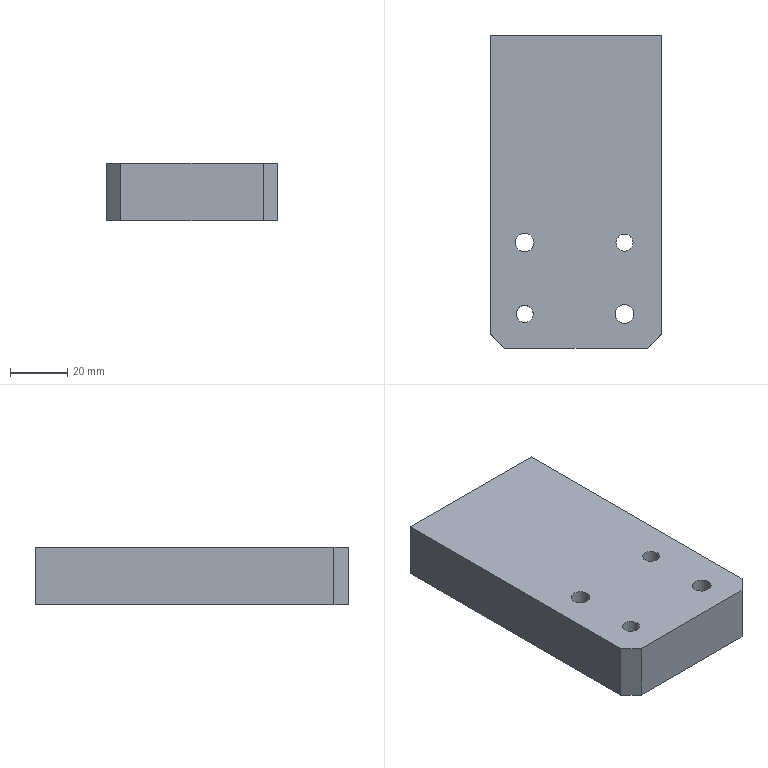Part | NX | features BREP 1 | 1 solid | 24 faces | box 60 x 109.5 x 20 mm | volume 126301 mm3 | plane 10 | cylinder 10 | cone 4 | commonest cylinder face diameters 6 x4 5 x2 6.6 x2 11 x2
STEP:
#1=CARTESIAN_POINT('',(30.,-49.75,-20.));
#2=VERTEX_POINT('',#1);
#3=CARTESIAN_POINT('',(30.,54.75,-20.));
#4=VERTEX_POINT('',#3);
#5=CARTESIAN_POINT('',(30.,54.75,-20.));
#6=DIRECTION('',(0.,1.,0.));
#7=VECTOR('',#6,1000.);
#8=LINE('',#5,#7);
#9=EDGE_CURVE('',#2,#4,#8,.T.);
#10=ORIENTED_EDGE('',*,*,#9,.T.);
#11=CARTESIAN_POINT('',(30.,54.75,0.));
#12=VERTEX_POINT('',#11);
#13=CARTESIAN_POINT('',(30.,54.75,-20.));
#14=DIRECTION('',(0.,0.,1.));
#15=VECTOR('',#14,1000.);
#16=LINE('',#13,#15);
#17=EDGE_CURVE('',#4,#12,#16,.T.);
#18=ORIENTED_EDGE('',*,*,#17,.T.);
#19=CARTESIAN_POINT('',(30.,-49.75,0.));
#20=VERTEX_POINT('',#19);
#21=CARTESIAN_POINT('',(30.,54.75,0.));
#22=DIRECTION('',(0.,1.,0.));
#23=VECTOR('',#22,1000.);
#24=LINE('',#21,#23);
#25=EDGE_CURVE('',#20,#12,#24,.T.);
#26=ORIENTED_EDGE('',*,*,#25,.F.);
#27=CARTESIAN_POINT('',(30.,-49.75,-20.));
#28=DIRECTION('',(0.,0.,1.));
#29=VECTOR('',#28,1000.);
#30=LINE('',#27,#29);
#31=EDGE_CURVE('',#2,#20,#30,.T.);
#32=ORIENTED_EDGE('',*,*,#31,.F.);
#33=EDGE_LOOP('',(#10,#18,#26,#32));
#34=FACE_BOUND('',#33,.T.);
#35=CARTESIAN_POINT('',(30.,54.75,-20.));
#36=DIRECTION('',(-1.,0.,0.));
#37=DIRECTION('',(0.,1.,0.));
#38=AXIS2_PLACEMENT_3D('',#35,#36,#37);
#39=PLANE('',#38);
#40=ADVANCED_FACE('',(#34),#39,.F.);
#41=CARTESIAN_POINT('',(-11.5,54.75,-13.));
#42=VERTEX_POINT('',#41);
#43=CARTESIAN_POINT('',(-11.5,54.75,-10.));
#44=DIRECTION('',(0.,-1.,0.));
#45=DIRECTION('',(0.,0.,-1.));
#46=AXIS2_PLACEMENT_3D('',#43,#44,#45);
#47=CIRCLE('',#46,3.);
#48=EDGE_CURVE('',#42,#42,#47,.T.);
#49=ORIENTED_EDGE('',*,*,#48,.T.);
#50=EDGE_LOOP('',(#49));
#51=FACE_BOUND('',#50,.T.);
#52=CARTESIAN_POINT('',(11.5,54.75,-13.));
#53=VERTEX_POINT('',#52);
#54=CARTESIAN_POINT('',(11.5,54.75,-10.));
#55=DIRECTION('',(0.,-1.,0.));
#56=DIRECTION('',(0.,0.,-1.));
#57=AXIS2_PLACEMENT_3D('',#54,#55,#56);
#58=CIRCLE('',#57,3.);
#59=EDGE_CURVE('',#53,#53,#58,.T.);
#60=ORIENTED_EDGE('',*,*,#59,.T.);
#61=EDGE_LOOP('',(#60));
#62=FACE_BOUND('',#61,.T.);
#63=CARTESIAN_POINT('',(-22.5,54.75,-12.5));
#64=VERTEX_POINT('',#63);
#65=CARTESIAN_POINT('',(-22.5,54.75,-10.));
#66=DIRECTION('',(0.,-1.,0.));
#67=DIRECTION('',(0.,0.,-1.));
#68=AXIS2_PLACEMENT_3D('',#65,#66,#67);
#69=CIRCLE('',#68,2.5);
#70=EDGE_CURVE('',#64,#64,#69,.T.);
#71=ORIENTED_EDGE('',*,*,#70,.T.);
#72=EDGE_LOOP('',(#71));
#73=FACE_BOUND('',#72,.T.);
#74=CARTESIAN_POINT('',(22.5,54.75,-12.5));
#75=VERTEX_POINT('',#74);
#76=CARTESIAN_POINT('',(22.5,54.75,-10.));
#77=DIRECTION('',(0.,-1.,0.));
#78=DIRECTION('',(0.,0.,-1.));
#79=AXIS2_PLACEMENT_3D('',#76,#77,#78);
#80=CIRCLE('',#79,2.5);
#81=EDGE_CURVE('',#75,#75,#80,.T.);
#82=ORIENTED_EDGE('',*,*,#81,.T.);
#83=EDGE_LOOP('',(#82));
#84=FACE_BOUND('',#83,.T.);
#85=CARTESIAN_POINT('',(-30.,54.75,0.));
#86=VERTEX_POINT('',#85);
#87=CARTESIAN_POINT('',(-30.,54.75,0.));
#88=DIRECTION('',(-1.,0.,0.));
#89=VECTOR('',#88,1000.);
#90=LINE('',#87,#89);
#91=EDGE_CURVE('',#12,#86,#90,.T.);
#92=ORIENTED_EDGE('',*,*,#91,.F.);
#93=ORIENTED_EDGE('',*,*,#17,.F.);
#94=CARTESIAN_POINT('',(-30.,54.75,-20.));
#95=VERTEX_POINT('',#94);
#96=CARTESIAN_POINT('',(-30.,54.75,-20.));
#97=DIRECTION('',(-1.,0.,0.));
#98=VECTOR('',#97,1000.);
#99=LINE('',#96,#98);
#100=EDGE_CURVE('',#4,#95,#99,.T.);
#101=ORIENTED_EDGE('',*,*,#100,.T.);
#102=CARTESIAN_POINT('',(-30.,54.75,-20.));
#103=DIRECTION('',(0.,0.,1.));
#104=VECTOR('',#103,1000.);
#105=LINE('',#102,#104);
#106=EDGE_CURVE('',#95,#86,#105,.T.);
#107=ORIENTED_EDGE('',*,*,#106,.T.);
#108=EDGE_LOOP('',(#92,#93,#101,#107));
#109=FACE_BOUND('',#108,.T.);
#110=CARTESIAN_POINT('',(-30.,54.75,-20.));
#111=DIRECTION('',(0.,-1.,0.));
#112=DIRECTION('',(0.,0.,-1.));
#113=AXIS2_PLACEMENT_3D('',#110,#111,#112);
#114=PLANE('',#113);
#115=ADVANCED_FACE('',(#51,#62,#73,#84,#109),#114,.F.);
#116=CARTESIAN_POINT('',(-30.,-49.75,0.));
#117=VERTEX_POINT('',#116);
#118=CARTESIAN_POINT('',(-30.,54.75,0.));
#119=DIRECTION('',(0.,-1.,0.));
#120=VECTOR('',#119,1000.);
#121=LINE('',#118,#120);
#122=EDGE_CURVE('',#86,#117,#121,.T.);
#123=ORIENTED_EDGE('',*,*,#122,.F.);
#124=ORIENTED_EDGE('',*,*,#106,.F.);
#125=CARTESIAN_POINT('',(-30.,-49.75,-20.));
#126=VERTEX_POINT('',#125);
#127=CARTESIAN_POINT('',(-30.,54.75,-20.));
#128=DIRECTION('',(0.,-1.,0.));
#129=VECTOR('',#128,1000.);
#130=LINE('',#127,#129);
#131=EDGE_CURVE('',#95,#126,#130,.T.);
#132=ORIENTED_EDGE('',*,*,#131,.T.);
#133=CARTESIAN_POINT('',(-30.,-49.75,-20.));
#134=DIRECTION('',(0.,0.,-1.));
#135=VECTOR('',#134,1000.);
#136=LINE('',#133,#135);
#137=EDGE_CURVE('',#117,#126,#136,.T.);
#138=ORIENTED_EDGE('',*,*,#137,.F.);
#139=EDGE_LOOP('',(#123,#124,#132,#138));
#140=FACE_BOUND('',#139,.T.);
#141=CARTESIAN_POINT('',(-30.,54.75,-20.));
#142=DIRECTION('',(1.,0.,0.));
#143=DIRECTION('',(0.,-1.,0.));
#144=AXIS2_PLACEMENT_3D('',#141,#142,#143);
#145=PLANE('',#144);
#146=ADVANCED_FACE('',(#140),#145,.F.);
#147=CARTESIAN_POINT('',(-25.,-54.75,0.));
#148=VERTEX_POINT('',#147);
#149=CARTESIAN_POINT('',(25.,-54.75,0.));
#150=VERTEX_POINT('',#149);
#151=CARTESIAN_POINT('',(-30.,-54.75,0.));
#152=DIRECTION('',(1.,0.,0.));
#153=VECTOR('',#152,1000.);
#154=LINE('',#151,#153);
#155=EDGE_CURVE('',#148,#150,#154,.T.);
#156=ORIENTED_EDGE('',*,*,#155,.F.);
#157=CARTESIAN_POINT('',(-25.,-54.75,-20.));
#158=VERTEX_POINT('',#157);
#159=CARTESIAN_POINT('',(-25.,-54.75,-20.));
#160=DIRECTION('',(0.,0.,1.));
#161=VECTOR('',#160,1000.);
#162=LINE('',#159,#161);
#163=EDGE_CURVE('',#158,#148,#162,.T.);
#164=ORIENTED_EDGE('',*,*,#163,.F.);
#165=CARTESIAN_POINT('',(25.,-54.75,-20.));
#166=VERTEX_POINT('',#165);
#167=CARTESIAN_POINT('',(-30.,-54.75,-20.));
#168=DIRECTION('',(1.,0.,0.));
#169=VECTOR('',#168,1000.);
#170=LINE('',#167,#169);
#171=EDGE_CURVE('',#158,#166,#170,.T.);
#172=ORIENTED_EDGE('',*,*,#171,.T.);
#173=CARTESIAN_POINT('',(25.,-54.75,-20.));
#174=DIRECTION('',(0.,0.,-1.));
#175=VECTOR('',#174,1000.);
#176=LINE('',#173,#175);
#177=EDGE_CURVE('',#150,#166,#176,.T.);
#178=ORIENTED_EDGE('',*,*,#177,.F.);
#179=EDGE_LOOP('',(#156,#164,#172,#178));
#180=FACE_BOUND('',#179,.T.);
#181=CARTESIAN_POINT('',(-30.,-54.75,-20.));
#182=DIRECTION('',(0.,1.,0.));
#183=DIRECTION('',(0.,0.,1.));
#184=AXIS2_PLACEMENT_3D('',#181,#182,#183);
#185=PLANE('',#184);
#186=ADVANCED_FACE('',(#180),#185,.F.);
#187=CARTESIAN_POINT('',(22.5,-42.75,-20.));
#188=VERTEX_POINT('',#187);
#189=CARTESIAN_POINT('',(17.,-42.75,-20.));
#190=DIRECTION('',(0.,0.,1.));
#191=DIRECTION('',(1.,0.,0.));
#192=AXIS2_PLACEMENT_3D('',#189,#190,#191);
#193=CIRCLE('',#192,5.5);
#194=EDGE_CURVE('',#188,#188,#193,.T.);
#195=ORIENTED_EDGE('',*,*,#194,.T.);
#196=EDGE_LOOP('',(#195));
#197=FACE_BOUND('',#196,.T.);
#198=CARTESIAN_POINT('',(-12.5,-17.75,-20.));
#199=VERTEX_POINT('',#198);
#200=CARTESIAN_POINT('',(-18.,-17.75,-20.));
#201=DIRECTION('',(0.,0.,1.));
#202=DIRECTION('',(1.,0.,0.));
#203=AXIS2_PLACEMENT_3D('',#200,#201,#202);
#204=CIRCLE('',#203,5.5);
#205=EDGE_CURVE('',#199,#199,#204,.T.);
#206=ORIENTED_EDGE('',*,*,#205,.T.);
#207=EDGE_LOOP('',(#206));
#208=FACE_BOUND('',#207,.T.);
#209=CARTESIAN_POINT('',(14.,-17.75,-20.));
#210=VERTEX_POINT('',#209);
#211=CARTESIAN_POINT('',(17.,-17.75,-20.));
#212=DIRECTION('',(0.,0.,-1.));
#213=DIRECTION('',(-1.,0.,0.));
#214=AXIS2_PLACEMENT_3D('',#211,#212,#213);
#215=CIRCLE('',#214,3.);
#216=EDGE_CURVE('',#210,#210,#215,.T.);
#217=ORIENTED_EDGE('',*,*,#216,.F.);
#218=EDGE_LOOP('',(#217));
#219=FACE_BOUND('',#218,.T.);
#220=CARTESIAN_POINT('',(-21.,-42.75,-20.));
#221=VERTEX_POINT('',#220);
#222=CARTESIAN_POINT('',(-18.,-42.75,-20.));
#223=DIRECTION('',(0.,0.,-1.));
#224=DIRECTION('',(-1.,0.,0.));
#225=AXIS2_PLACEMENT_3D('',#222,#223,#224);
#226=CIRCLE('',#225,3.);
#227=EDGE_CURVE('',#221,#221,#226,.T.);
#228=ORIENTED_EDGE('',*,*,#227,.F.);
#229=EDGE_LOOP('',(#228));
#230=FACE_BOUND('',#229,.T.);
#231=ORIENTED_EDGE('',*,*,#171,.F.);
#232=CARTESIAN_POINT('',(-39.875,-39.875,-20.));
#233=DIRECTION('',(0.7071,-0.7071,0.));
#234=VECTOR('',#233,1000.);
#235=LINE('',#232,#234);
#236=EDGE_CURVE('',#126,#158,#235,.T.);
#237=ORIENTED_EDGE('',*,*,#236,.F.);
#238=ORIENTED_EDGE('',*,*,#131,.F.);
#239=ORIENTED_EDGE('',*,*,#100,.F.);
#240=ORIENTED_EDGE('',*,*,#9,.F.);
#241=CARTESIAN_POINT('',(39.875,-39.875,-20.));
#242=DIRECTION('',(0.7071,0.7071,0.));
#243=VECTOR('',#242,1000.);
#244=LINE('',#241,#243);
#245=EDGE_CURVE('',#166,#2,#244,.T.);
#246=ORIENTED_EDGE('',*,*,#245,.F.);
#247=EDGE_LOOP('',(#231,#237,#238,#239,#240,#246));
#248=FACE_BOUND('',#247,.T.);
#249=CARTESIAN_POINT('',(0.,0.,-20.));
#250=DIRECTION('',(0.,0.,-1.));
#251=DIRECTION('',(-1.,0.,0.));
#252=AXIS2_PLACEMENT_3D('',#249,#250,#251);
#253=PLANE('',#252);
#254=ADVANCED_FACE('',(#197,#208,#219,#230,#248),#253,.T.);
#255=CARTESIAN_POINT('',(20.3,-42.75,0.));
#256=VERTEX_POINT('',#255);
#257=CARTESIAN_POINT('',(17.,-42.75,0.));
#258=DIRECTION('',(0.,0.,1.));
#259=DIRECTION('',(1.,0.,0.));
#260=AXIS2_PLACEMENT_3D('',#257,#258,#259);
#261=CIRCLE('',#260,3.3);
#262=EDGE_CURVE('',#256,#256,#261,.T.);
#263=ORIENTED_EDGE('',*,*,#262,.F.);
#264=EDGE_LOOP('',(#263));
#265=FACE_BOUND('',#264,.T.);
#266=CARTESIAN_POINT('',(-14.7,-17.75,0.));
#267=VERTEX_POINT('',#266);
#268=CARTESIAN_POINT('',(-18.,-17.75,0.));
#269=DIRECTION('',(0.,0.,1.));
#270=DIRECTION('',(1.,0.,0.));
#271=AXIS2_PLACEMENT_3D('',#268,#269,#270);
#272=CIRCLE('',#271,3.3);
#273=EDGE_CURVE('',#267,#267,#272,.T.);
#274=ORIENTED_EDGE('',*,*,#273,.F.);
#275=EDGE_LOOP('',(#274));
#276=FACE_BOUND('',#275,.T.);
#277=CARTESIAN_POINT('',(14.,-17.75,0.));
#278=VERTEX_POINT('',#277);
#279=CARTESIAN_POINT('',(17.,-17.75,0.));
#280=DIRECTION('',(0.,0.,-1.));
#281=DIRECTION('',(-1.,0.,0.));
#282=AXIS2_PLACEMENT_3D('',#279,#280,#281);
#283=CIRCLE('',#282,3.);
#284=EDGE_CURVE('',#278,#278,#283,.T.);
#285=ORIENTED_EDGE('',*,*,#284,.T.);
#286=EDGE_LOOP('',(#285));
#287=FACE_BOUND('',#286,.T.);
#288=CARTESIAN_POINT('',(-21.,-42.75,0.));
#289=VERTEX_POINT('',#288);
#290=CARTESIAN_POINT('',(-18.,-42.75,0.));
#291=DIRECTION('',(0.,0.,-1.));
#292=DIRECTION('',(-1.,0.,0.));
#293=AXIS2_PLACEMENT_3D('',#290,#291,#292);
#294=CIRCLE('',#293,3.);
#295=EDGE_CURVE('',#289,#289,#294,.T.);
#296=ORIENTED_EDGE('',*,*,#295,.T.);
#297=EDGE_LOOP('',(#296));
#298=FACE_BOUND('',#297,.T.);
#299=ORIENTED_EDGE('',*,*,#25,.T.);
#300=ORIENTED_EDGE('',*,*,#91,.T.);
#301=ORIENTED_EDGE('',*,*,#122,.T.);
#302=CARTESIAN_POINT('',(-25.,-54.75,0.));
#303=DIRECTION('',(-0.7071,0.7071,0.));
#304=VECTOR('',#303,1000.);
#305=LINE('',#302,#304);
#306=EDGE_CURVE('',#148,#117,#305,.T.);
#307=ORIENTED_EDGE('',*,*,#306,.F.);
#308=ORIENTED_EDGE('',*,*,#155,.T.);
#309=CARTESIAN_POINT('',(30.,-49.75,0.));
#310=DIRECTION('',(-0.7071,-0.7071,0.));
#311=VECTOR('',#310,1000.);
#312=LINE('',#309,#311);
#313=EDGE_CURVE('',#20,#150,#312,.T.);
#314=ORIENTED_EDGE('',*,*,#313,.F.);
#315=EDGE_LOOP('',(#299,#300,#301,#307,#308,#314));
#316=FACE_BOUND('',#315,.T.);
#317=CARTESIAN_POINT('',(0.,0.,0.));
#318=DIRECTION('',(0.,0.,-1.));
#319=DIRECTION('',(-1.,0.,0.));
#320=AXIS2_PLACEMENT_3D('',#317,#318,#319);
#321=PLANE('',#320);
#322=ADVANCED_FACE('',(#265,#276,#287,#298,#316),#321,.F.);
#323=ORIENTED_EDGE('',*,*,#227,.T.);
#324=EDGE_LOOP('',(#323));
#325=FACE_BOUND('',#324,.T.);
#326=ORIENTED_EDGE('',*,*,#295,.F.);
#327=EDGE_LOOP('',(#326));
#328=FACE_BOUND('',#327,.T.);
#329=CARTESIAN_POINT('',(-18.,-42.75,0.));
#330=DIRECTION('',(0.,0.,1.));
#331=DIRECTION('',(1.,0.,0.));
#332=AXIS2_PLACEMENT_3D('',#329,#330,#331);
#333=CYLINDRICAL_SURFACE('',#332,3.);
#334=ADVANCED_FACE('',(#325,#328),#333,.F.);
#335=ORIENTED_EDGE('',*,*,#216,.T.);
#336=EDGE_LOOP('',(#335));
#337=FACE_BOUND('',#336,.T.);
#338=ORIENTED_EDGE('',*,*,#284,.F.);
#339=EDGE_LOOP('',(#338));
#340=FACE_BOUND('',#339,.T.);
#341=CARTESIAN_POINT('',(17.,-17.75,0.));
#342=DIRECTION('',(0.,0.,1.));
#343=DIRECTION('',(1.,0.,0.));
#344=AXIS2_PLACEMENT_3D('',#341,#342,#343);
#345=CYLINDRICAL_SURFACE('',#344,3.);
#346=ADVANCED_FACE('',(#337,#340),#345,.F.);
#347=ORIENTED_EDGE('',*,*,#273,.T.);
#348=EDGE_LOOP('',(#347));
#349=FACE_BOUND('',#348,.T.);
#350=CARTESIAN_POINT('',(-14.7,-17.75,-13.6));
#351=VERTEX_POINT('',#350);
#352=CARTESIAN_POINT('',(-18.,-17.75,-13.6));
#353=DIRECTION('',(0.,0.,1.));
#354=DIRECTION('',(1.,0.,0.));
#355=AXIS2_PLACEMENT_3D('',#352,#353,#354);
#356=CIRCLE('',#355,3.3);
#357=EDGE_CURVE('',#351,#351,#356,.T.);
#358=ORIENTED_EDGE('',*,*,#357,.F.);
#359=EDGE_LOOP('',(#358));
#360=FACE_BOUND('',#359,.T.);
#361=CARTESIAN_POINT('',(-18.,-17.75,-20.));
#362=DIRECTION('',(0.,0.,-1.));
#363=DIRECTION('',(-1.,0.,0.));
#364=AXIS2_PLACEMENT_3D('',#361,#362,#363);
#365=CYLINDRICAL_SURFACE('',#364,3.3);
#366=ADVANCED_FACE('',(#349,#360),#365,.F.);
#367=ORIENTED_EDGE('',*,*,#357,.T.);
#368=EDGE_LOOP('',(#367));
#369=FACE_BOUND('',#368,.T.);
#370=CARTESIAN_POINT('',(-12.5,-17.75,-13.6));
#371=VERTEX_POINT('',#370);
#372=CARTESIAN_POINT('',(-18.,-17.75,-13.6));
#373=DIRECTION('',(0.,0.,1.));
#374=DIRECTION('',(1.,0.,0.));
#375=AXIS2_PLACEMENT_3D('',#372,#373,#374);
#376=CIRCLE('',#375,5.5);
#377=EDGE_CURVE('',#371,#371,#376,.T.);
#378=ORIENTED_EDGE('',*,*,#377,.F.);
#379=EDGE_LOOP('',(#378));
#380=FACE_BOUND('',#379,.T.);
#381=CARTESIAN_POINT('',(-14.7,-17.75,-13.6));
#382=DIRECTION('',(0.,0.,1.));
#383=DIRECTION('',(1.,0.,0.));
#384=AXIS2_PLACEMENT_3D('',#381,#382,#383);
#385=PLANE('',#384);
#386=ADVANCED_FACE('',(#369,#380),#385,.F.);
#387=ORIENTED_EDGE('',*,*,#377,.T.);
#388=EDGE_LOOP('',(#387));
#389=FACE_BOUND('',#388,.T.);
#390=ORIENTED_EDGE('',*,*,#205,.F.);
#391=EDGE_LOOP('',(#390));
#392=FACE_BOUND('',#391,.T.);
#393=CARTESIAN_POINT('',(-18.,-17.75,-20.));
#394=DIRECTION('',(0.,0.,-1.));
#395=DIRECTION('',(-1.,0.,0.));
#396=AXIS2_PLACEMENT_3D('',#393,#394,#395);
#397=CYLINDRICAL_SURFACE('',#396,5.5);
#398=ADVANCED_FACE('',(#389,#392),#397,.F.);
#399=ORIENTED_EDGE('',*,*,#262,.T.);
#400=EDGE_LOOP('',(#399));
#401=FACE_BOUND('',#400,.T.);
#402=CARTESIAN_POINT('',(20.3,-42.75,-13.6));
#403=VERTEX_POINT('',#402);
#404=CARTESIAN_POINT('',(17.,-42.75,-13.6));
#405=DIRECTION('',(0.,0.,1.));
#406=DIRECTION('',(1.,0.,0.));
#407=AXIS2_PLACEMENT_3D('',#404,#405,#406);
#408=CIRCLE('',#407,3.3);
#409=EDGE_CURVE('',#403,#403,#408,.T.);
#410=ORIENTED_EDGE('',*,*,#409,.F.);
#411=EDGE_LOOP('',(#410));
#412=FACE_BOUND('',#411,.T.);
#413=CARTESIAN_POINT('',(17.,-42.75,-20.));
#414=DIRECTION('',(0.,0.,-1.));
#415=DIRECTION('',(-1.,0.,0.));
#416=AXIS2_PLACEMENT_3D('',#413,#414,#415);
#417=CYLINDRICAL_SURFACE('',#416,3.3);
#418=ADVANCED_FACE('',(#401,#412),#417,.F.);
#419=ORIENTED_EDGE('',*,*,#409,.T.);
#420=EDGE_LOOP('',(#419));
#421=FACE_BOUND('',#420,.T.);
#422=CARTESIAN_POINT('',(22.5,-42.75,-13.6));
#423=VERTEX_POINT('',#422);
#424=CARTESIAN_POINT('',(17.,-42.75,-13.6));
#425=DIRECTION('',(0.,0.,1.));
#426=DIRECTION('',(1.,0.,0.));
#427=AXIS2_PLACEMENT_3D('',#424,#425,#426);
#428=CIRCLE('',#427,5.5);
#429=EDGE_CURVE('',#423,#423,#428,.T.);
#430=ORIENTED_EDGE('',*,*,#429,.F.);
#431=EDGE_LOOP('',(#430));
#432=FACE_BOUND('',#431,.T.);
#433=CARTESIAN_POINT('',(20.3,-42.75,-13.6));
#434=DIRECTION('',(0.,0.,1.));
#435=DIRECTION('',(1.,0.,0.));
#436=AXIS2_PLACEMENT_3D('',#433,#434,#435);
#437=PLANE('',#436);
#438=ADVANCED_FACE('',(#421,#432),#437,.F.);
#439=ORIENTED_EDGE('',*,*,#429,.T.);
#440=EDGE_LOOP('',(#439));
#441=FACE_BOUND('',#440,.T.);
#442=ORIENTED_EDGE('',*,*,#194,.F.);
#443=EDGE_LOOP('',(#442));
#444=FACE_BOUND('',#443,.T.);
#445=CARTESIAN_POINT('',(17.,-42.75,-20.));
#446=DIRECTION('',(0.,0.,-1.));
#447=DIRECTION('',(-1.,0.,0.));
#448=AXIS2_PLACEMENT_3D('',#445,#446,#447);
#449=CYLINDRICAL_SURFACE('',#448,5.5);
#450=ADVANCED_FACE('',(#441,#444),#449,.F.);
#451=ORIENTED_EDGE('',*,*,#245,.T.);
#452=ORIENTED_EDGE('',*,*,#31,.T.);
#453=ORIENTED_EDGE('',*,*,#313,.T.);
#454=ORIENTED_EDGE('',*,*,#177,.T.);
#455=EDGE_LOOP('',(#451,#452,#453,#454));
#456=FACE_BOUND('',#455,.T.);
#457=CARTESIAN_POINT('',(30.,-49.75,-20.));
#458=DIRECTION('',(-0.7071,0.7071,0.));
#459=DIRECTION('',(0.,0.,-1.));
#460=AXIS2_PLACEMENT_3D('',#457,#458,#459);
#461=PLANE('',#460);
#462=ADVANCED_FACE('',(#456),#461,.F.);
#463=ORIENTED_EDGE('',*,*,#236,.T.);
#464=ORIENTED_EDGE('',*,*,#163,.T.);
#465=ORIENTED_EDGE('',*,*,#306,.T.);
#466=ORIENTED_EDGE('',*,*,#137,.T.);
#467=EDGE_LOOP('',(#463,#464,#465,#466));
#468=FACE_BOUND('',#467,.T.);
#469=CARTESIAN_POINT('',(-25.,-54.75,-20.));
#470=DIRECTION('',(0.7071,0.7071,0.));
#471=DIRECTION('',(0.,0.,-1.));
#472=AXIS2_PLACEMENT_3D('',#469,#470,#471);
#473=PLANE('',#472);
#474=ADVANCED_FACE('',(#468),#473,.F.);
#475=CARTESIAN_POINT('',(22.5,38.248,-10.));
#476=VERTEX_POINT('',#475);
#477=VERTEX_LOOP('',#476);
#478=FACE_BOUND('',#477,.T.);
#479=CARTESIAN_POINT('',(22.5,39.75,-12.5));
#480=VERTEX_POINT('',#479);
#481=CARTESIAN_POINT('',(22.5,39.75,-10.));
#482=DIRECTION('',(0.,-1.,0.));
#483=DIRECTION('',(0.,0.,-1.));
#484=AXIS2_PLACEMENT_3D('',#481,#482,#483);
#485=CIRCLE('',#484,2.5);
#486=EDGE_CURVE('',#480,#480,#485,.T.);
#487=ORIENTED_EDGE('',*,*,#486,.F.);
#488=EDGE_LOOP('',(#487));
#489=FACE_BOUND('',#488,.T.);
#490=CARTESIAN_POINT('',(22.5,39.75,-10.));
#491=DIRECTION('',(0.,1.,0.));
#492=DIRECTION('',(0.,0.,1.));
#493=AXIS2_PLACEMENT_3D('',#490,#491,#492);
#494=CONICAL_SURFACE('',#493,2.5,1.03);
#495=ADVANCED_FACE('',(#478,#489),#494,.F.);
#496=ORIENTED_EDGE('',*,*,#486,.T.);
#497=EDGE_LOOP('',(#496));
#498=FACE_BOUND('',#497,.T.);
#499=ORIENTED_EDGE('',*,*,#81,.F.);
#500=EDGE_LOOP('',(#499));
#501=FACE_BOUND('',#500,.T.);
#502=CARTESIAN_POINT('',(22.5,54.75,-10.));
#503=DIRECTION('',(0.,1.,0.));
#504=DIRECTION('',(0.,0.,1.));
#505=AXIS2_PLACEMENT_3D('',#502,#503,#504);
#506=CYLINDRICAL_SURFACE('',#505,2.5);
#507=ADVANCED_FACE('',(#498,#501),#506,.F.);
#508=CARTESIAN_POINT('',(-22.5,38.248,-10.));
#509=VERTEX_POINT('',#508);
#510=VERTEX_LOOP('',#509);
#511=FACE_BOUND('',#510,.T.);
#512=CARTESIAN_POINT('',(-22.5,39.75,-12.5));
#513=VERTEX_POINT('',#512);
#514=CARTESIAN_POINT('',(-22.5,39.75,-10.));
#515=DIRECTION('',(0.,-1.,0.));
#516=DIRECTION('',(0.,0.,-1.));
#517=AXIS2_PLACEMENT_3D('',#514,#515,#516);
#518=CIRCLE('',#517,2.5);
#519=EDGE_CURVE('',#513,#513,#518,.T.);
#520=ORIENTED_EDGE('',*,*,#519,.F.);
#521=EDGE_LOOP('',(#520));
#522=FACE_BOUND('',#521,.T.);
#523=CARTESIAN_POINT('',(-22.5,39.75,-10.));
#524=DIRECTION('',(0.,1.,0.));
#525=DIRECTION('',(0.,0.,1.));
#526=AXIS2_PLACEMENT_3D('',#523,#524,#525);
#527=CONICAL_SURFACE('',#526,2.5,1.03);
#528=ADVANCED_FACE('',(#511,#522),#527,.F.);
#529=ORIENTED_EDGE('',*,*,#519,.T.);
#530=EDGE_LOOP('',(#529));
#531=FACE_BOUND('',#530,.T.);
#532=ORIENTED_EDGE('',*,*,#70,.F.);
#533=EDGE_LOOP('',(#532));
#534=FACE_BOUND('',#533,.T.);
#535=CARTESIAN_POINT('',(-22.5,54.75,-10.));
#536=DIRECTION('',(0.,1.,0.));
#537=DIRECTION('',(0.,0.,1.));
#538=AXIS2_PLACEMENT_3D('',#535,#536,#537);
#539=CYLINDRICAL_SURFACE('',#538,2.5);
#540=ADVANCED_FACE('',(#531,#534),#539,.F.);
#541=CARTESIAN_POINT('',(11.5,40.947,-10.));
#542=VERTEX_POINT('',#541);
#543=VERTEX_LOOP('',#542);
#544=FACE_BOUND('',#543,.T.);
#545=CARTESIAN_POINT('',(11.5,42.75,-13.));
#546=VERTEX_POINT('',#545);
#547=CARTESIAN_POINT('',(11.5,42.75,-10.));
#548=DIRECTION('',(0.,-1.,0.));
#549=DIRECTION('',(0.,0.,-1.));
#550=AXIS2_PLACEMENT_3D('',#547,#548,#549);
#551=CIRCLE('',#550,3.);
#552=EDGE_CURVE('',#546,#546,#551,.T.);
#553=ORIENTED_EDGE('',*,*,#552,.F.);
#554=EDGE_LOOP('',(#553));
#555=FACE_BOUND('',#554,.T.);
#556=CARTESIAN_POINT('',(11.5,42.75,-10.));
#557=DIRECTION('',(0.,1.,0.));
#558=DIRECTION('',(0.,0.,1.));
#559=AXIS2_PLACEMENT_3D('',#556,#557,#558);
#560=CONICAL_SURFACE('',#559,3.,1.03);
#561=ADVANCED_FACE('',(#544,#555),#560,.F.);
#562=ORIENTED_EDGE('',*,*,#552,.T.);
#563=EDGE_LOOP('',(#562));
#564=FACE_BOUND('',#563,.T.);
#565=ORIENTED_EDGE('',*,*,#59,.F.);
#566=EDGE_LOOP('',(#565));
#567=FACE_BOUND('',#566,.T.);
#568=CARTESIAN_POINT('',(11.5,54.75,-10.));
#569=DIRECTION('',(0.,1.,0.));
#570=DIRECTION('',(0.,0.,1.));
#571=AXIS2_PLACEMENT_3D('',#568,#569,#570);
#572=CYLINDRICAL_SURFACE('',#571,3.);
#573=ADVANCED_FACE('',(#564,#567),#572,.F.);
#574=CARTESIAN_POINT('',(-11.5,40.947,-10.));
#575=VERTEX_POINT('',#574);
#576=VERTEX_LOOP('',#575);
#577=FACE_BOUND('',#576,.T.);
#578=CARTESIAN_POINT('',(-11.5,42.75,-13.));
#579=VERTEX_POINT('',#578);
#580=CARTESIAN_POINT('',(-11.5,42.75,-10.));
#581=DIRECTION('',(0.,-1.,0.));
#582=DIRECTION('',(0.,0.,-1.));
#583=AXIS2_PLACEMENT_3D('',#580,#581,#582);
#584=CIRCLE('',#583,3.);
#585=EDGE_CURVE('',#579,#579,#584,.T.);
#586=ORIENTED_EDGE('',*,*,#585,.F.);
#587=EDGE_LOOP('',(#586));
#588=FACE_BOUND('',#587,.T.);
#589=CARTESIAN_POINT('',(-11.5,42.75,-10.));
#590=DIRECTION('',(0.,1.,0.));
#591=DIRECTION('',(0.,0.,1.));
#592=AXIS2_PLACEMENT_3D('',#589,#590,#591);
#593=CONICAL_SURFACE('',#592,3.,1.03);
#594=ADVANCED_FACE('',(#577,#588),#593,.F.);
#595=ORIENTED_EDGE('',*,*,#585,.T.);
#596=EDGE_LOOP('',(#595));
#597=FACE_BOUND('',#596,.T.);
#598=ORIENTED_EDGE('',*,*,#48,.F.);
#599=EDGE_LOOP('',(#598));
#600=FACE_BOUND('',#599,.T.);
#601=CARTESIAN_POINT('',(-11.5,54.75,-10.));
#602=DIRECTION('',(0.,1.,0.));
#603=DIRECTION('',(0.,0.,1.));
#604=AXIS2_PLACEMENT_3D('',#601,#602,#603);
#605=CYLINDRICAL_SURFACE('',#604,3.);
#606=ADVANCED_FACE('',(#597,#600),#605,.F.);
#607=CLOSED_SHELL('',(#40,#115,#146,#186,#254,#322,#334,#346,#366,#386,#398,#418,#438,#450,#462,#474,#495,#507,#528,#540,#561,#573,#594,#606));
#608=MANIFOLD_SOLID_BREP('',#607);
#609=(LENGTH_UNIT()NAMED_UNIT(*)SI_UNIT(.MILLI.,.METRE.));
#610=UNCERTAINTY_MEASURE_WITH_UNIT(LENGTH_MEASURE(0.00001),#609,'','');
#611=(NAMED_UNIT(*)PLANE_ANGLE_UNIT()SI_UNIT($,.RADIAN.));
#612=(NAMED_UNIT(*)SI_UNIT($,.STERADIAN.)SOLID_ANGLE_UNIT());
#613=(GEOMETRIC_REPRESENTATION_CONTEXT(3)GLOBAL_UNCERTAINTY_ASSIGNED_CONTEXT((#610))GLOBAL_UNIT_ASSIGNED_CONTEXT((#609,#611,#612))REPRESENTATION_CONTEXT('',''));
#614=ADVANCED_BREP_SHAPE_REPRESENTATION('',(#608),#613);